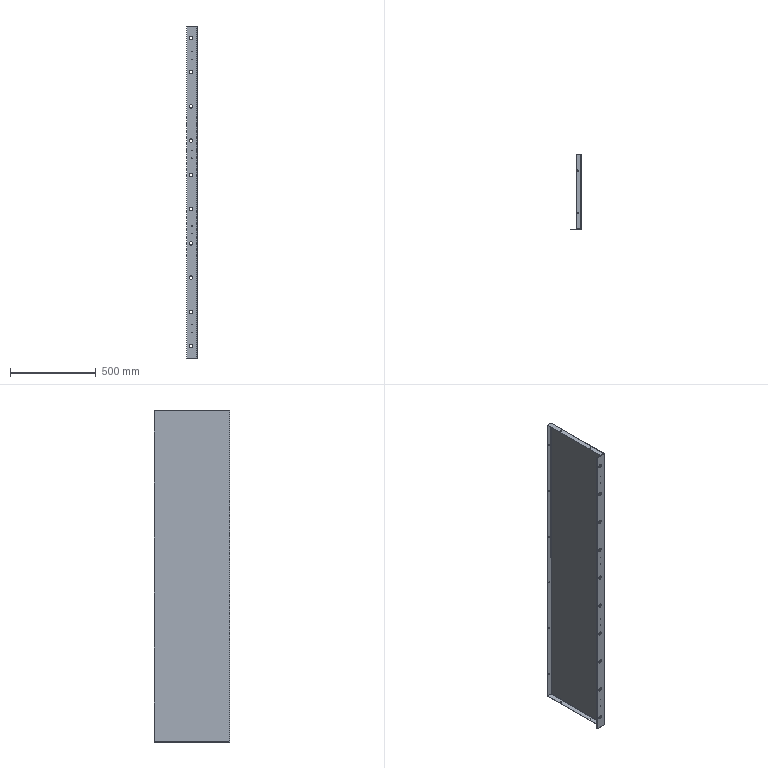Part | STEP file | JBJ-P-1011-04 | 1 solid | 98 faces | box 61.5 x 440 x 1940 mm | volume 1252283 mm3 | plane 58 | cylinder 36 | spline 4 | commonest cylinder face diameters 6.5 x10 20.5 x10 3.5 x8 2.4 x4 4.8 x4